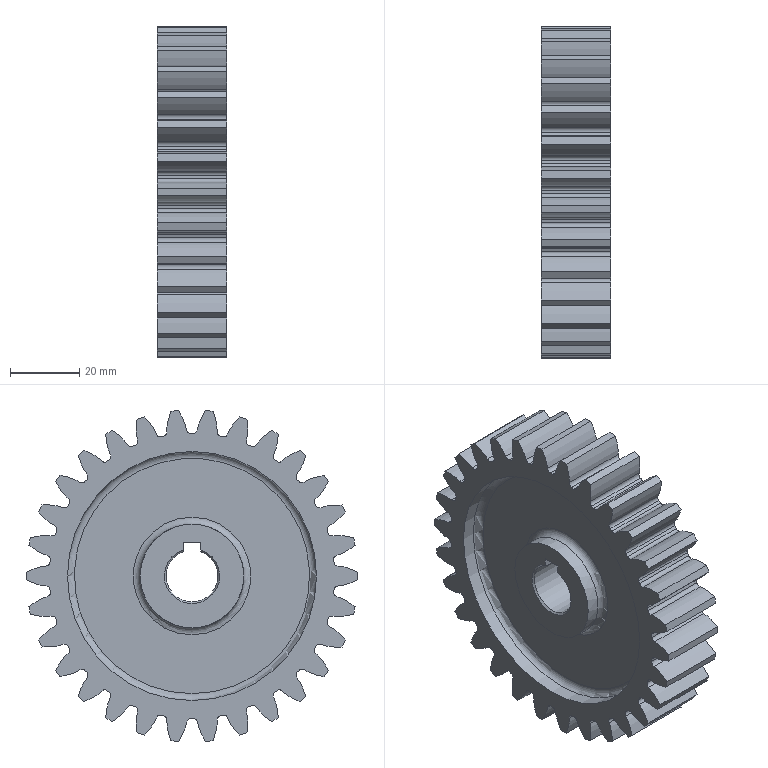Part | NX | features BREP 30, META 30, EXTRUDE 3, DATUM_CSYS 2, EXTRACT_FACE 2, EXTRACT_STRING 2, BLEND 1, CHAMFER 1, CYLINDER 1, DATUM_PLANE 1, FSET 1, Instance Feature 1, Mirror Feature 1, SKETCH 1 | 1 solid | 200 faces | box 20 x 96 x 95.68 mm | volume 82292 mm3 | spline 150 | cylinder 35 | plane 9 | torus 4 | cone 2 | commonest cylinder face diameters 82.5 x30 30 x2 72 x2 15 x1